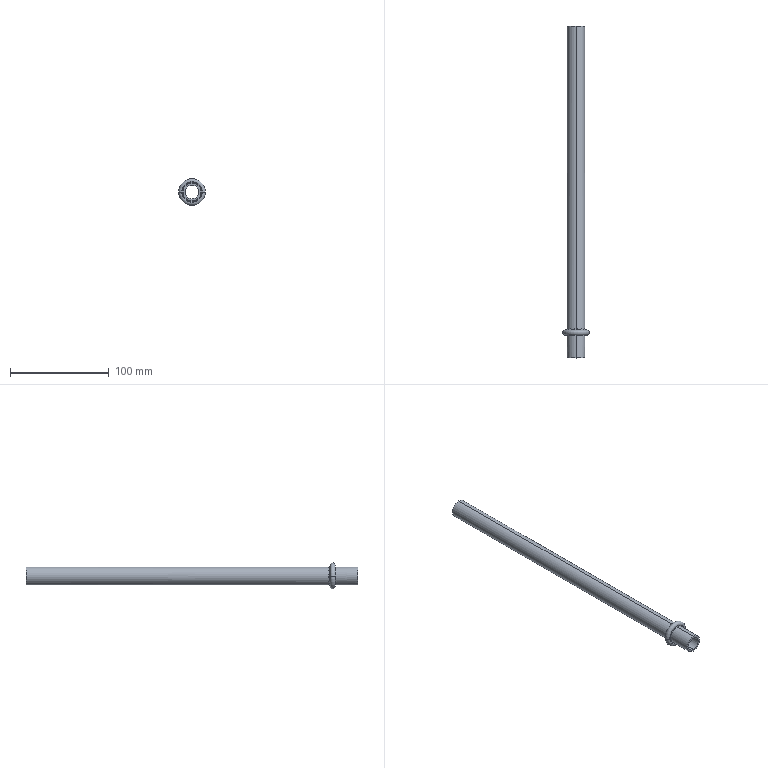Part | NX | features BREP 1 | 1 solid | 38 faces | box 27 x 335.45 x 27 mm | volume 34706 mm3 | torus 20 | cone 8 | cylinder 8 | plane 2 | commonest cylinder face diameters 14 x4 18 x4
STEP:
#1=CARTESIAN_POINT('',(-290.548,-139.151,-153.339));
#2=VERTEX_POINT('',#1);
#3=CARTESIAN_POINT('',(-289.046,-143.915,-153.339));
#4=VERTEX_POINT('',#3);
#5=CARTESIAN_POINT('',(-289.693,-141.5,-153.339));
#6=DIRECTION('',(0.,0.,1.));
#7=DIRECTION('',(1.,0.,0.));
#8=AXIS2_PLACEMENT_3D('',#5,#6,#7);
#9=CIRCLE('',#8,2.5);
#10=EDGE_CURVE('',#2,#4,#9,.T.);
#11=ORIENTED_EDGE('',*,*,#10,.T.);
#12=CARTESIAN_POINT('',(-268.34,-143.915,-153.339));
#13=VERTEX_POINT('',#12);
#14=CARTESIAN_POINT('',(-278.693,-143.915,-153.339));
#15=DIRECTION('',(0.,-1.,0.));
#16=DIRECTION('',(1.,0.,0.));
#17=AXIS2_PLACEMENT_3D('',#14,#15,#16);
#18=CIRCLE('',#17,10.353);
#19=EDGE_CURVE('',#13,#4,#18,.T.);
#20=ORIENTED_EDGE('',*,*,#19,.F.);
#21=CARTESIAN_POINT('',(-266.838,-139.151,-153.339));
#22=VERTEX_POINT('',#21);
#23=CARTESIAN_POINT('',(-267.693,-141.5,-153.339));
#24=DIRECTION('',(0.,0.,-1.));
#25=DIRECTION('',(-1.,0.,0.));
#26=AXIS2_PLACEMENT_3D('',#23,#24,#25);
#27=CIRCLE('',#26,2.5);
#28=EDGE_CURVE('',#22,#13,#27,.T.);
#29=ORIENTED_EDGE('',*,*,#28,.F.);
#30=CARTESIAN_POINT('',(-278.693,-139.151,-153.339));
#31=DIRECTION('',(0.,-1.,0.));
#32=DIRECTION('',(1.,0.,0.));
#33=AXIS2_PLACEMENT_3D('',#30,#31,#32);
#34=CIRCLE('',#33,11.855);
#35=EDGE_CURVE('',#22,#2,#34,.T.);
#36=ORIENTED_EDGE('',*,*,#35,.T.);
#37=EDGE_LOOP('',(#11,#20,#29,#36));
#38=FACE_BOUND('',#37,.T.);
#39=CARTESIAN_POINT('',(-278.693,-141.5,-153.339));
#40=DIRECTION('',(0.,-1.,0.));
#41=DIRECTION('',(-1.,0.,0.));
#42=AXIS2_PLACEMENT_3D('',#39,#40,#41);
#43=TOROIDAL_SURFACE('',#42,11.,2.5);
#44=ADVANCED_FACE('',(#38),#43,.T.);
#45=ORIENTED_EDGE('',*,*,#28,.T.);
#46=CARTESIAN_POINT('',(-278.693,-143.915,-153.339));
#47=DIRECTION('',(0.,-1.,0.));
#48=DIRECTION('',(-1.,0.,0.));
#49=AXIS2_PLACEMENT_3D('',#46,#47,#48);
#50=CIRCLE('',#49,10.353);
#51=EDGE_CURVE('',#4,#13,#50,.T.);
#52=ORIENTED_EDGE('',*,*,#51,.F.);
#53=ORIENTED_EDGE('',*,*,#10,.F.);
#54=CARTESIAN_POINT('',(-278.693,-139.151,-153.339));
#55=DIRECTION('',(0.,-1.,0.));
#56=DIRECTION('',(-1.,0.,0.));
#57=AXIS2_PLACEMENT_3D('',#54,#55,#56);
#58=CIRCLE('',#57,11.855);
#59=EDGE_CURVE('',#2,#22,#58,.T.);
#60=ORIENTED_EDGE('',*,*,#59,.T.);
#61=EDGE_LOOP('',(#45,#52,#53,#60));
#62=FACE_BOUND('',#61,.T.);
#63=CARTESIAN_POINT('',(-278.693,-141.5,-153.339));
#64=DIRECTION('',(0.,-1.,0.));
#65=DIRECTION('',(1.,0.,0.));
#66=AXIS2_PLACEMENT_3D('',#63,#64,#65);
#67=TOROIDAL_SURFACE('',#66,11.,2.5);
#68=ADVANCED_FACE('',(#62),#67,.T.);
#69=CARTESIAN_POINT('',(-288.351,-138.351,-153.339));
#70=VERTEX_POINT('',#69);
#71=CARTESIAN_POINT('',(-288.351,-138.351,-153.339));
#72=DIRECTION('',(-0.9397,-0.342,0.));
#73=VECTOR('',#72,1000.);
#74=LINE('',#71,#73);
#75=EDGE_CURVE('',#70,#2,#74,.T.);
#76=ORIENTED_EDGE('',*,*,#75,.T.);
#77=ORIENTED_EDGE('',*,*,#35,.F.);
#78=CARTESIAN_POINT('',(-269.035,-138.351,-153.339));
#79=VERTEX_POINT('',#78);
#80=CARTESIAN_POINT('',(-269.035,-138.351,-153.339));
#81=DIRECTION('',(0.9397,-0.342,0.));
#82=VECTOR('',#81,1000.);
#83=LINE('',#80,#82);
#84=EDGE_CURVE('',#79,#22,#83,.T.);
#85=ORIENTED_EDGE('',*,*,#84,.F.);
#86=CARTESIAN_POINT('',(-278.693,-138.351,-143.681));
#87=VERTEX_POINT('',#86);
#88=CARTESIAN_POINT('',(-278.693,-138.351,-153.339));
#89=DIRECTION('',(0.,-1.,0.));
#90=DIRECTION('',(1.,0.,0.));
#91=AXIS2_PLACEMENT_3D('',#88,#89,#90);
#92=CIRCLE('',#91,9.658);
#93=EDGE_CURVE('',#79,#87,#92,.T.);
#94=ORIENTED_EDGE('',*,*,#93,.T.);
#95=CARTESIAN_POINT('',(-278.693,-138.351,-153.339));
#96=DIRECTION('',(0.,-1.,0.));
#97=DIRECTION('',(0.,0.,1.));
#98=AXIS2_PLACEMENT_3D('',#95,#96,#97);
#99=CIRCLE('',#98,9.658);
#100=EDGE_CURVE('',#87,#70,#99,.T.);
#101=ORIENTED_EDGE('',*,*,#100,.T.);
#102=EDGE_LOOP('',(#76,#77,#85,#94,#101));
#103=FACE_BOUND('',#102,.T.);
#104=CARTESIAN_POINT('',(-278.693,-138.351,-153.339));
#105=DIRECTION('',(0.,-1.,0.));
#106=DIRECTION('',(0.,0.,1.));
#107=AXIS2_PLACEMENT_3D('',#104,#105,#106);
#108=CONICAL_SURFACE('',#107,9.658,1.222);
#109=ADVANCED_FACE('',(#103),#108,.T.);
#110=ORIENTED_EDGE('',*,*,#84,.T.);
#111=ORIENTED_EDGE('',*,*,#59,.F.);
#112=ORIENTED_EDGE('',*,*,#75,.F.);
#113=CARTESIAN_POINT('',(-278.693,-138.351,-162.997));
#114=VERTEX_POINT('',#113);
#115=CARTESIAN_POINT('',(-278.693,-138.351,-153.339));
#116=DIRECTION('',(0.,-1.,0.));
#117=DIRECTION('',(-1.,0.,0.));
#118=AXIS2_PLACEMENT_3D('',#115,#116,#117);
#119=CIRCLE('',#118,9.658);
#120=EDGE_CURVE('',#70,#114,#119,.T.);
#121=ORIENTED_EDGE('',*,*,#120,.T.);
#122=CARTESIAN_POINT('',(-278.693,-138.351,-153.339));
#123=DIRECTION('',(0.,-1.,0.));
#124=DIRECTION('',(0.,0.,-1.));
#125=AXIS2_PLACEMENT_3D('',#122,#123,#124);
#126=CIRCLE('',#125,9.658);
#127=EDGE_CURVE('',#114,#79,#126,.T.);
#128=ORIENTED_EDGE('',*,*,#127,.T.);
#129=EDGE_LOOP('',(#110,#111,#112,#121,#128));
#130=FACE_BOUND('',#129,.T.);
#131=CARTESIAN_POINT('',(-278.693,-138.351,-153.339));
#132=DIRECTION('',(0.,-1.,0.));
#133=DIRECTION('',(0.,0.,-1.));
#134=AXIS2_PLACEMENT_3D('',#131,#132,#133);
#135=CONICAL_SURFACE('',#134,9.658,1.222);
#136=ADVANCED_FACE('',(#130),#135,.T.);
#137=CARTESIAN_POINT('',(-278.693,-137.411,-144.339));
#138=VERTEX_POINT('',#137);
#139=CARTESIAN_POINT('',(-278.693,168.3,-144.339));
#140=VERTEX_POINT('',#139);
#141=CARTESIAN_POINT('',(-278.693,-137.411,-144.339));
#142=DIRECTION('',(0.,1.,0.));
#143=VECTOR('',#142,1000.);
#144=LINE('',#141,#143);
#145=EDGE_CURVE('',#138,#140,#144,.T.);
#146=ORIENTED_EDGE('',*,*,#145,.F.);
#147=CARTESIAN_POINT('',(-269.693,-137.411,-153.339));
#148=VERTEX_POINT('',#147);
#149=CARTESIAN_POINT('',(-278.693,-137.411,-153.339));
#150=DIRECTION('',(0.,-1.,0.));
#151=DIRECTION('',(1.,0.,0.));
#152=AXIS2_PLACEMENT_3D('',#149,#150,#151);
#153=CIRCLE('',#152,9.);
#154=EDGE_CURVE('',#148,#138,#153,.T.);
#155=ORIENTED_EDGE('',*,*,#154,.F.);
#156=CARTESIAN_POINT('',(-278.693,-137.411,-162.339));
#157=VERTEX_POINT('',#156);
#158=CARTESIAN_POINT('',(-278.693,-137.411,-153.339));
#159=DIRECTION('',(0.,-1.,0.));
#160=DIRECTION('',(0.,0.,-1.));
#161=AXIS2_PLACEMENT_3D('',#158,#159,#160);
#162=CIRCLE('',#161,9.);
#163=EDGE_CURVE('',#157,#148,#162,.T.);
#164=ORIENTED_EDGE('',*,*,#163,.F.);
#165=CARTESIAN_POINT('',(-278.693,168.3,-162.339));
#166=VERTEX_POINT('',#165);
#167=CARTESIAN_POINT('',(-278.693,-137.411,-162.339));
#168=DIRECTION('',(0.,1.,0.));
#169=VECTOR('',#168,1000.);
#170=LINE('',#167,#169);
#171=EDGE_CURVE('',#157,#166,#170,.T.);
#172=ORIENTED_EDGE('',*,*,#171,.T.);
#173=CARTESIAN_POINT('',(-278.693,168.3,-153.339));
#174=DIRECTION('',(0.,1.,0.));
#175=DIRECTION('',(0.,0.,1.));
#176=AXIS2_PLACEMENT_3D('',#173,#174,#175);
#177=CIRCLE('',#176,9.);
#178=EDGE_CURVE('',#140,#166,#177,.T.);
#179=ORIENTED_EDGE('',*,*,#178,.F.);
#180=EDGE_LOOP('',(#146,#155,#164,#172,#179));
#181=FACE_BOUND('',#180,.T.);
#182=CARTESIAN_POINT('',(-278.693,-137.411,-153.339));
#183=DIRECTION('',(0.,1.,0.));
#184=DIRECTION('',(0.,0.,-1.));
#185=AXIS2_PLACEMENT_3D('',#182,#183,#184);
#186=CYLINDRICAL_SURFACE('',#185,9.);
#187=ADVANCED_FACE('',(#181),#186,.T.);
#188=ORIENTED_EDGE('',*,*,#145,.T.);
#189=CARTESIAN_POINT('',(-278.693,168.3,-153.339));
#190=DIRECTION('',(0.,1.,0.));
#191=DIRECTION('',(0.,0.,-1.));
#192=AXIS2_PLACEMENT_3D('',#189,#190,#191);
#193=CIRCLE('',#192,9.);
#194=EDGE_CURVE('',#166,#140,#193,.T.);
#195=ORIENTED_EDGE('',*,*,#194,.F.);
#196=ORIENTED_EDGE('',*,*,#171,.F.);
#197=CARTESIAN_POINT('',(-287.693,-137.411,-153.339));
#198=VERTEX_POINT('',#197);
#199=CARTESIAN_POINT('',(-278.693,-137.411,-153.339));
#200=DIRECTION('',(0.,-1.,0.));
#201=DIRECTION('',(-1.,0.,0.));
#202=AXIS2_PLACEMENT_3D('',#199,#200,#201);
#203=CIRCLE('',#202,9.);
#204=EDGE_CURVE('',#198,#157,#203,.T.);
#205=ORIENTED_EDGE('',*,*,#204,.F.);
#206=CARTESIAN_POINT('',(-278.693,-137.411,-153.339));
#207=DIRECTION('',(0.,-1.,0.));
#208=DIRECTION('',(0.,0.,1.));
#209=AXIS2_PLACEMENT_3D('',#206,#207,#208);
#210=CIRCLE('',#209,9.);
#211=EDGE_CURVE('',#138,#198,#210,.T.);
#212=ORIENTED_EDGE('',*,*,#211,.F.);
#213=EDGE_LOOP('',(#188,#195,#196,#205,#212));
#214=FACE_BOUND('',#213,.T.);
#215=CARTESIAN_POINT('',(-278.693,-137.411,-153.339));
#216=DIRECTION('',(0.,1.,0.));
#217=DIRECTION('',(0.,0.,-1.));
#218=AXIS2_PLACEMENT_3D('',#215,#216,#217);
#219=CYLINDRICAL_SURFACE('',#218,9.);
#220=ADVANCED_FACE('',(#214),#219,.T.);
#221=CARTESIAN_POINT('',(-268.693,-137.411,-153.339));
#222=DIRECTION('',(0.,0.,1.));
#223=DIRECTION('',(0.,-1.,0.));
#224=AXIS2_PLACEMENT_3D('',#221,#222,#223);
#225=CIRCLE('',#224,1.);
#226=EDGE_CURVE('',#148,#79,#225,.T.);
#227=ORIENTED_EDGE('',*,*,#226,.F.);
#228=ORIENTED_EDGE('',*,*,#154,.T.);
#229=CARTESIAN_POINT('',(-278.693,-137.411,-143.339));
#230=DIRECTION('',(-1.,0.,0.));
#231=DIRECTION('',(0.,0.,1.));
#232=AXIS2_PLACEMENT_3D('',#229,#230,#231);
#233=CIRCLE('',#232,1.);
#234=EDGE_CURVE('',#138,#87,#233,.T.);
#235=ORIENTED_EDGE('',*,*,#234,.T.);
#236=ORIENTED_EDGE('',*,*,#93,.F.);
#237=EDGE_LOOP('',(#227,#228,#235,#236));
#238=FACE_BOUND('',#237,.T.);
#239=CARTESIAN_POINT('',(-278.693,-137.411,-153.339));
#240=DIRECTION('',(0.,1.,0.));
#241=DIRECTION('',(0.,0.,-1.));
#242=AXIS2_PLACEMENT_3D('',#239,#240,#241);
#243=TOROIDAL_SURFACE('',#242,10.,1.);
#244=ADVANCED_FACE('',(#238),#243,.F.);
#245=ORIENTED_EDGE('',*,*,#234,.F.);
#246=ORIENTED_EDGE('',*,*,#211,.T.);
#247=CARTESIAN_POINT('',(-288.693,-137.411,-153.339));
#248=DIRECTION('',(0.,0.,-1.));
#249=DIRECTION('',(0.,1.,0.));
#250=AXIS2_PLACEMENT_3D('',#247,#248,#249);
#251=CIRCLE('',#250,1.);
#252=EDGE_CURVE('',#198,#70,#251,.T.);
#253=ORIENTED_EDGE('',*,*,#252,.T.);
#254=ORIENTED_EDGE('',*,*,#100,.F.);
#255=EDGE_LOOP('',(#245,#246,#253,#254));
#256=FACE_BOUND('',#255,.T.);
#257=CARTESIAN_POINT('',(-278.693,-137.411,-153.339));
#258=DIRECTION('',(0.,-1.,0.));
#259=DIRECTION('',(0.,0.,-1.));
#260=AXIS2_PLACEMENT_3D('',#257,#258,#259);
#261=TOROIDAL_SURFACE('',#260,10.,1.);
#262=ADVANCED_FACE('',(#256),#261,.F.);
#263=ORIENTED_EDGE('',*,*,#252,.F.);
#264=ORIENTED_EDGE('',*,*,#204,.T.);
#265=CARTESIAN_POINT('',(-278.693,-137.411,-163.339));
#266=DIRECTION('',(1.,0.,0.));
#267=DIRECTION('',(0.,1.,0.));
#268=AXIS2_PLACEMENT_3D('',#265,#266,#267);
#269=CIRCLE('',#268,1.);
#270=EDGE_CURVE('',#157,#114,#269,.T.);
#271=ORIENTED_EDGE('',*,*,#270,.T.);
#272=ORIENTED_EDGE('',*,*,#120,.F.);
#273=EDGE_LOOP('',(#263,#264,#271,#272));
#274=FACE_BOUND('',#273,.T.);
#275=CARTESIAN_POINT('',(-278.693,-137.411,-153.339));
#276=DIRECTION('',(0.,1.,0.));
#277=DIRECTION('',(0.,0.,1.));
#278=AXIS2_PLACEMENT_3D('',#275,#276,#277);
#279=TOROIDAL_SURFACE('',#278,10.,1.);
#280=ADVANCED_FACE('',(#274),#279,.F.);
#281=ORIENTED_EDGE('',*,*,#270,.F.);
#282=ORIENTED_EDGE('',*,*,#163,.T.);
#283=ORIENTED_EDGE('',*,*,#226,.T.);
#284=ORIENTED_EDGE('',*,*,#127,.F.);
#285=EDGE_LOOP('',(#281,#282,#283,#284));
#286=FACE_BOUND('',#285,.T.);
#287=CARTESIAN_POINT('',(-278.693,-137.411,-153.339));
#288=DIRECTION('',(0.,1.,0.));
#289=DIRECTION('',(-1.,0.,0.));
#290=AXIS2_PLACEMENT_3D('',#287,#288,#289);
#291=TOROIDAL_SURFACE('',#290,10.,1.);
#292=ADVANCED_FACE('',(#286),#291,.F.);
#293=CARTESIAN_POINT('',(-288.071,-143.653,-153.339));
#294=VERTEX_POINT('',#293);
#295=CARTESIAN_POINT('',(-289.046,-143.915,-153.339));
#296=DIRECTION('',(0.9659,0.2588,0.));
#297=VECTOR('',#296,1000.);
#298=LINE('',#295,#297);
#299=EDGE_CURVE('',#4,#294,#298,.T.);
#300=ORIENTED_EDGE('',*,*,#299,.T.);
#301=CARTESIAN_POINT('',(-278.693,-143.653,-143.961));
#302=VERTEX_POINT('',#301);
#303=CARTESIAN_POINT('',(-278.693,-143.653,-153.339));
#304=DIRECTION('',(0.,-1.,0.));
#305=DIRECTION('',(0.,0.,1.));
#306=AXIS2_PLACEMENT_3D('',#303,#304,#305);
#307=CIRCLE('',#306,9.378);
#308=EDGE_CURVE('',#302,#294,#307,.T.);
#309=ORIENTED_EDGE('',*,*,#308,.F.);
#310=CARTESIAN_POINT('',(-269.315,-143.653,-153.339));
#311=VERTEX_POINT('',#310);
#312=CARTESIAN_POINT('',(-278.693,-143.653,-153.339));
#313=DIRECTION('',(0.,-1.,0.));
#314=DIRECTION('',(1.,0.,0.));
#315=AXIS2_PLACEMENT_3D('',#312,#313,#314);
#316=CIRCLE('',#315,9.378);
#317=EDGE_CURVE('',#311,#302,#316,.T.);
#318=ORIENTED_EDGE('',*,*,#317,.F.);
#319=CARTESIAN_POINT('',(-268.34,-143.915,-153.339));
#320=DIRECTION('',(-0.9659,0.2588,0.));
#321=VECTOR('',#320,1000.);
#322=LINE('',#319,#321);
#323=EDGE_CURVE('',#13,#311,#322,.T.);
#324=ORIENTED_EDGE('',*,*,#323,.F.);
#325=ORIENTED_EDGE('',*,*,#19,.T.);
#326=EDGE_LOOP('',(#300,#309,#318,#324,#325));
#327=FACE_BOUND('',#326,.T.);
#328=CARTESIAN_POINT('',(-278.693,-143.653,-153.339));
#329=DIRECTION('',(0.,-1.,0.));
#330=DIRECTION('',(0.,0.,1.));
#331=AXIS2_PLACEMENT_3D('',#328,#329,#330);
#332=CONICAL_SURFACE('',#331,9.378,1.309);
#333=ADVANCED_FACE('',(#327),#332,.F.);
#334=ORIENTED_EDGE('',*,*,#323,.T.);
#335=CARTESIAN_POINT('',(-278.693,-143.653,-162.717));
#336=VERTEX_POINT('',#335);
#337=CARTESIAN_POINT('',(-278.693,-143.653,-153.339));
#338=DIRECTION('',(0.,-1.,0.));
#339=DIRECTION('',(0.,0.,-1.));
#340=AXIS2_PLACEMENT_3D('',#337,#338,#339);
#341=CIRCLE('',#340,9.378);
#342=EDGE_CURVE('',#336,#311,#341,.T.);
#343=ORIENTED_EDGE('',*,*,#342,.F.);
#344=CARTESIAN_POINT('',(-278.693,-143.653,-153.339));
#345=DIRECTION('',(0.,-1.,0.));
#346=DIRECTION('',(-1.,0.,0.));
#347=AXIS2_PLACEMENT_3D('',#344,#345,#346);
#348=CIRCLE('',#347,9.378);
#349=EDGE_CURVE('',#294,#336,#348,.T.);
#350=ORIENTED_EDGE('',*,*,#349,.F.);
#351=ORIENTED_EDGE('',*,*,#299,.F.);
#352=ORIENTED_EDGE('',*,*,#51,.T.);
#353=EDGE_LOOP('',(#334,#343,#350,#351,#352));
#354=FACE_BOUND('',#353,.T.);
#355=CARTESIAN_POINT('',(-278.693,-143.653,-153.339));
#356=DIRECTION('',(0.,-1.,0.));
#357=DIRECTION('',(0.,0.,-1.));
#358=AXIS2_PLACEMENT_3D('',#355,#356,#357);
#359=CONICAL_SURFACE('',#358,9.378,1.309);
#360=ADVANCED_FACE('',(#354),#359,.F.);
#361=CARTESIAN_POINT('',(-278.693,-167.15,-144.339));
#362=VERTEX_POINT('',#361);
#363=CARTESIAN_POINT('',(-278.693,-143.943,-144.339));
#364=VERTEX_POINT('',#363);
#365=CARTESIAN_POINT('',(-278.693,-167.15,-144.339));
#366=DIRECTION('',(0.,1.,0.));
#367=VECTOR('',#366,1000.);
#368=LINE('',#365,#367);
#369=EDGE_CURVE('',#362,#364,#368,.T.);
#370=ORIENTED_EDGE('',*,*,#369,.F.);
#371=CARTESIAN_POINT('',(-278.693,-167.15,-162.339));
#372=VERTEX_POINT('',#371);
#373=CARTESIAN_POINT('',(-278.693,-167.15,-153.339));
#374=DIRECTION('',(0.,1.,0.));
#375=DIRECTION('',(0.,0.,1.));
#376=AXIS2_PLACEMENT_3D('',#373,#374,#375);
#377=CIRCLE('',#376,9.);
#378=EDGE_CURVE('',#362,#372,#377,.T.);
#379=ORIENTED_EDGE('',*,*,#378,.T.);
#380=CARTESIAN_POINT('',(-278.693,-143.943,-162.339));
#381=VERTEX_POINT('',#380);
#382=CARTESIAN_POINT('',(-278.693,-167.15,-162.339));
#383=DIRECTION('',(0.,1.,0.));
#384=VECTOR('',#383,1000.);
#385=LINE('',#382,#384);
#386=EDGE_CURVE('',#372,#381,#385,.T.);
#387=ORIENTED_EDGE('',*,*,#386,.T.);
#388=CARTESIAN_POINT('',(-269.693,-143.943,-153.339));
#389=VERTEX_POINT('',#388);
#390=CARTESIAN_POINT('',(-278.693,-143.943,-153.339));
#391=DIRECTION('',(0.,-1.,0.));
#392=DIRECTION('',(0.,0.,-1.));
#393=AXIS2_PLACEMENT_3D('',#390,#391,#392);
#394=CIRCLE('',#393,9.);
#395=EDGE_CURVE('',#381,#389,#394,.T.);
#396=ORIENTED_EDGE('',*,*,#395,.T.);
#397=CARTESIAN_POINT('',(-278.693,-143.943,-153.339));
#398=DIRECTION('',(0.,-1.,0.));
#399=DIRECTION('',(1.,0.,0.));
#400=AXIS2_PLACEMENT_3D('',#397,#398,#399);
#401=CIRCLE('',#400,9.);
#402=EDGE_CURVE('',#389,#364,#401,.T.);
#403=ORIENTED_EDGE('',*,*,#402,.T.);
#404=EDGE_LOOP('',(#370,#379,#387,#396,#403));
#405=FACE_BOUND('',#404,.T.);
#406=CARTESIAN_POINT('',(-278.693,-167.15,-153.339));
#407=DIRECTION('',(0.,1.,0.));
#408=DIRECTION('',(0.,0.,-1.));
#409=AXIS2_PLACEMENT_3D('',#406,#407,#408);
#410=CYLINDRICAL_SURFACE('',#409,9.);
#411=ADVANCED_FACE('',(#405),#410,.T.);
#412=ORIENTED_EDGE('',*,*,#369,.T.);
#413=CARTESIAN_POINT('',(-287.693,-143.943,-153.339));
#414=VERTEX_POINT('',#413);
#415=CARTESIAN_POINT('',(-278.693,-143.943,-153.339));
#416=DIRECTION('',(0.,-1.,0.));
#417=DIRECTION('',(0.,0.,1.));
#418=AXIS2_PLACEMENT_3D('',#415,#416,#417);
#419=CIRCLE('',#418,9.);
#420=EDGE_CURVE('',#364,#414,#419,.T.);
#421=ORIENTED_EDGE('',*,*,#420,.T.);
#422=CARTESIAN_POINT('',(-278.693,-143.943,-153.339));
#423=DIRECTION('',(0.,-1.,0.));
#424=DIRECTION('',(-1.,0.,0.));
#425=AXIS2_PLACEMENT_3D('',#422,#423,#424);
#426=CIRCLE('',#425,9.);
#427=EDGE_CURVE('',#414,#381,#426,.T.);
#428=ORIENTED_EDGE('',*,*,#427,.T.);
#429=ORIENTED_EDGE('',*,*,#386,.F.);
#430=CARTESIAN_POINT('',(-278.693,-167.15,-153.339));
#431=DIRECTION('',(0.,1.,0.));
#432=DIRECTION('',(0.,0.,-1.));
#433=AXIS2_PLACEMENT_3D('',#430,#431,#432);
#434=CIRCLE('',#433,9.);
#435=EDGE_CURVE('',#372,#362,#434,.T.);
#436=ORIENTED_EDGE('',*,*,#435,.T.);
#437=EDGE_LOOP('',(#412,#421,#428,#429,#436));
#438=FACE_BOUND('',#437,.T.);
#439=CARTESIAN_POINT('',(-278.693,-167.15,-153.339));
#440=DIRECTION('',(0.,1.,0.));
#441=DIRECTION('',(0.,0.,-1.));
#442=AXIS2_PLACEMENT_3D('',#439,#440,#441);
#443=CYLINDRICAL_SURFACE('',#442,9.);
#444=ADVANCED_FACE('',(#438),#443,.T.);
#445=CARTESIAN_POINT('',(-269.393,-143.943,-153.339));
#446=DIRECTION('',(0.,0.,-1.));
#447=DIRECTION('',(-1.,0.,0.));
#448=AXIS2_PLACEMENT_3D('',#445,#446,#447);
#449=CIRCLE('',#448,0.3);
#450=EDGE_CURVE('',#311,#389,#449,.F.);
#451=ORIENTED_EDGE('',*,*,#450,.F.);
#452=ORIENTED_EDGE('',*,*,#317,.T.);
#453=CARTESIAN_POINT('',(-278.693,-143.943,-144.039));
#454=DIRECTION('',(1.,0.,0.));
#455=DIRECTION('',(0.,0.,-1.));
#456=AXIS2_PLACEMENT_3D('',#453,#454,#455);
#457=CIRCLE('',#456,0.3);
#458=EDGE_CURVE('',#302,#364,#457,.F.);
#459=ORIENTED_EDGE('',*,*,#458,.T.);
#460=ORIENTED_EDGE('',*,*,#402,.F.);
#461=EDGE_LOOP('',(#451,#452,#459,#460));
#462=FACE_BOUND('',#461,.T.);
#463=CARTESIAN_POINT('',(-278.693,-143.943,-153.339));
#464=DIRECTION('',(0.,-1.,0.));
#465=DIRECTION('',(-1.,0.,0.));
#466=AXIS2_PLACEMENT_3D('',#463,#464,#465);
#467=TOROIDAL_SURFACE('',#466,9.3,0.3);
#468=ADVANCED_FACE('',(#462),#467,.F.);
#469=ORIENTED_EDGE('',*,*,#458,.F.);
#470=ORIENTED_EDGE('',*,*,#308,.T.);
#471=CARTESIAN_POINT('',(-287.993,-143.943,-153.339));
#472=DIRECTION('',(0.,0.,1.));
#473=DIRECTION('',(1.,0.,0.));
#474=AXIS2_PLACEMENT_3D('',#471,#472,#473);
#475=CIRCLE('',#474,0.3);
#476=EDGE_CURVE('',#294,#414,#475,.F.);
#477=ORIENTED_EDGE('',*,*,#476,.T.);
#478=ORIENTED_EDGE('',*,*,#420,.F.);
#479=EDGE_LOOP('',(#469,#470,#477,#478));
#480=FACE_BOUND('',#479,.T.);
#481=CARTESIAN_POINT('',(-278.693,-143.943,-153.339));
#482=DIRECTION('',(0.,-1.,0.));
#483=DIRECTION('',(0.,0.,-1.));
#484=AXIS2_PLACEMENT_3D('',#481,#482,#483);
#485=TOROIDAL_SURFACE('',#484,9.3,0.3);
#486=ADVANCED_FACE('',(#480),#485,.F.);
#487=ORIENTED_EDGE('',*,*,#476,.F.);
#488=ORIENTED_EDGE('',*,*,#349,.T.);
#489=CARTESIAN_POINT('',(-278.693,-143.943,-162.639));
#490=DIRECTION('',(-1.,0.,0.));
#491=DIRECTION('',(0.,0.,1.));
#492=AXIS2_PLACEMENT_3D('',#489,#490,#491);
#493=CIRCLE('',#492,0.3);
#494=EDGE_CURVE('',#336,#381,#493,.F.);
#495=ORIENTED_EDGE('',*,*,#494,.T.);
#496=ORIENTED_EDGE('',*,*,#427,.F.);
#497=EDGE_LOOP('',(#487,#488,#495,#496));
#498=FACE_BOUND('',#497,.T.);
#499=CARTESIAN_POINT('',(-278.693,-143.943,-153.339));
#500=DIRECTION('',(0.,-1.,0.));
#501=DIRECTION('',(1.,0.,0.));
#502=AXIS2_PLACEMENT_3D('',#499,#500,#501);
#503=TOROIDAL_SURFACE('',#502,9.3,0.3);
#504=ADVANCED_FACE('',(#498),#503,.F.);
#505=ORIENTED_EDGE('',*,*,#494,.F.);
#506=ORIENTED_EDGE('',*,*,#342,.T.);
#507=ORIENTED_EDGE('',*,*,#450,.T.);
#508=ORIENTED_EDGE('',*,*,#395,.F.);
#509=EDGE_LOOP('',(#505,#506,#507,#508));
#510=FACE_BOUND('',#509,.T.);
#511=CARTESIAN_POINT('',(-278.693,-143.943,-153.339));
#512=DIRECTION('',(0.,-1.,0.));
#513=DIRECTION('',(0.,0.,1.));
#514=AXIS2_PLACEMENT_3D('',#511,#512,#513);
#515=TOROIDAL_SURFACE('',#514,9.3,0.3);
#516=ADVANCED_FACE('',(#510),#515,.F.);
#517=ORIENTED_EDGE('',*,*,#178,.T.);
#518=ORIENTED_EDGE('',*,*,#194,.T.);
#519=EDGE_LOOP('',(#517,#518));
#520=FACE_BOUND('',#519,.T.);
#521=CARTESIAN_POINT('',(-278.693,168.3,-160.339));
#522=VERTEX_POINT('',#521);
#523=CARTESIAN_POINT('',(-278.693,168.3,-146.339));
#524=VERTEX_POINT('',#523);
#525=CARTESIAN_POINT('',(-278.693,168.3,-153.339));
#526=DIRECTION('',(0.,-1.,0.));
#527=DIRECTION('',(0.,0.,-1.));
#528=AXIS2_PLACEMENT_3D('',#525,#526,#527);
#529=CIRCLE('',#528,7.);
#530=EDGE_CURVE('',#522,#524,#529,.T.);
#531=ORIENTED_EDGE('',*,*,#530,.T.);
#532=CARTESIAN_POINT('',(-278.693,168.3,-153.339));
#533=DIRECTION('',(0.,-1.,0.));
#534=DIRECTION('',(0.,0.,1.));
#535=AXIS2_PLACEMENT_3D('',#532,#533,#534);
#536=CIRCLE('',#535,7.);
#537=EDGE_CURVE('',#524,#522,#536,.T.);
#538=ORIENTED_EDGE('',*,*,#537,.T.);
#539=EDGE_LOOP('',(#531,#538));
#540=FACE_BOUND('',#539,.T.);
#541=CARTESIAN_POINT('',(-294.893,168.3,-164.139));
#542=DIRECTION('',(0.,1.,0.));
#543=DIRECTION('',(-1.,0.,0.));
#544=AXIS2_PLACEMENT_3D('',#541,#542,#543);
#545=PLANE('',#544);
#546=ADVANCED_FACE('',(#520,#540),#545,.T.);
#547=ORIENTED_EDGE('',*,*,#378,.F.);
#548=ORIENTED_EDGE('',*,*,#435,.F.);
#549=EDGE_LOOP('',(#547,#548));
#550=FACE_BOUND('',#549,.T.);
#551=CARTESIAN_POINT('',(-278.693,-167.15,-160.339));
#552=VERTEX_POINT('',#551);
#553=CARTESIAN_POINT('',(-278.693,-167.15,-146.339));
#554=VERTEX_POINT('',#553);
#555=CARTESIAN_POINT('',(-278.693,-167.15,-153.339));
#556=DIRECTION('',(0.,1.,0.));
#557=DIRECTION('',(0.,0.,-1.));
#558=AXIS2_PLACEMENT_3D('',#555,#556,#557);
#559=CIRCLE('',#558,7.);
#560=EDGE_CURVE('',#552,#554,#559,.T.);
#561=ORIENTED_EDGE('',*,*,#560,.T.);
#562=CARTESIAN_POINT('',(-278.693,-167.15,-153.339));
#563=DIRECTION('',(0.,1.,0.));
#564=DIRECTION('',(0.,0.,1.));
#565=AXIS2_PLACEMENT_3D('',#562,#563,#564);
#566=CIRCLE('',#565,7.);
#567=EDGE_CURVE('',#554,#552,#566,.T.);
#568=ORIENTED_EDGE('',*,*,#567,.T.);
#569=EDGE_LOOP('',(#561,#568));
#570=FACE_BOUND('',#569,.T.);
#571=CARTESIAN_POINT('',(-294.893,-167.15,-164.139));
#572=DIRECTION('',(0.,-1.,0.));
#573=DIRECTION('',(0.,0.,1.));
#574=AXIS2_PLACEMENT_3D('',#571,#572,#573);
#575=PLANE('',#574);
#576=ADVANCED_FACE('',(#550,#570),#575,.T.);
#577=CARTESIAN_POINT('',(-271.693,-137.411,-153.339));
#578=VERTEX_POINT('',#577);
#579=CARTESIAN_POINT('',(-278.693,-137.411,-160.339));
#580=VERTEX_POINT('',#579);
#581=CARTESIAN_POINT('',(-278.693,-137.411,-160.339));
#582=CARTESIAN_POINT('',(-276.86,-137.411,-160.339));
#583=CARTESIAN_POINT('',(-273.21,-137.411,-158.822));
#584=CARTESIAN_POINT('',(-271.693,-137.411,-155.172));
#585=CARTESIAN_POINT('',(-271.693,-137.411,-153.339));
#586=B_SPLINE_CURVE_WITH_KNOTS('',3,(#581,#582,#583,#584,#585),.UNSPECIFIED.,.F.,.F.,(4,1,4),(0.,0.5,1.),.UNSPECIFIED.);
#587=EDGE_CURVE('',#578,#580,#586,.F.);
#588=ORIENTED_EDGE('',*,*,#587,.T.);
#589=CARTESIAN_POINT('',(-278.693,-140.23,-162.313));
#590=VERTEX_POINT('',#589);
#591=CARTESIAN_POINT('',(-278.693,-140.23,-162.313));
#592=CARTESIAN_POINT('',(-278.693,-139.813,-161.165));
#593=CARTESIAN_POINT('',(-278.693,-138.633,-160.339));
#594=CARTESIAN_POINT('',(-278.693,-137.411,-160.339));
#595=B_SPLINE_CURVE_WITH_KNOTS('',3,(#591,#592,#593,#594),.UNSPECIFIED.,.F.,.F.,(4,4),(0.,1.),.UNSPECIFIED.);
#596=EDGE_CURVE('',#590,#580,#595,.T.);
#597=ORIENTED_EDGE('',*,*,#596,.F.);
#598=CARTESIAN_POINT('',(-269.719,-140.23,-153.339));
#599=VERTEX_POINT('',#598);
#600=CARTESIAN_POINT('',(-278.693,-140.23,-162.313));
#601=CARTESIAN_POINT('',(-276.344,-140.23,-162.313));
#602=CARTESIAN_POINT('',(-271.664,-140.23,-160.368));
#603=CARTESIAN_POINT('',(-269.719,-140.23,-155.688));
#604=CARTESIAN_POINT('',(-269.719,-140.23,-153.339));
#605=B_SPLINE_CURVE_WITH_KNOTS('',3,(#600,#601,#602,#603,#604),.UNSPECIFIED.,.F.,.F.,(4,1,4),(0.,0.5,1.),.UNSPECIFIED.);
#606=EDGE_CURVE('',#599,#590,#605,.F.);
#607=ORIENTED_EDGE('',*,*,#606,.F.);
#608=CARTESIAN_POINT('',(-269.719,-140.23,-153.339));
#609=CARTESIAN_POINT('',(-270.867,-139.813,-153.339));
#610=CARTESIAN_POINT('',(-271.693,-138.633,-153.339));
#611=CARTESIAN_POINT('',(-271.693,-137.411,-153.339));
#612=B_SPLINE_CURVE_WITH_KNOTS('',3,(#608,#609,#610,#611),.UNSPECIFIED.,.F.,.F.,(4,4),(0.,1.),.UNSPECIFIED.);
#613=EDGE_CURVE('',#599,#578,#612,.T.);
#614=ORIENTED_EDGE('',*,*,#613,.T.);
#615=EDGE_LOOP('',(#588,#597,#607,#614));
#616=FACE_BOUND('',#615,.T.);
#617=CARTESIAN_POINT('',(-278.694,-137.411,-153.338));
#618=DIRECTION('',(0.,1.,0.));
#619=DIRECTION('',(-1.,0.,0.00006098));
#620=AXIS2_PLACEMENT_3D('',#617,#618,#619);
#621=TOROIDAL_SURFACE('',#620,10.001,3.);
#622=ADVANCED_FACE('',(#616),#621,.T.);
#623=CARTESIAN_POINT('',(-278.693,-137.411,-146.339));
#624=VERTEX_POINT('',#623);
#625=CARTESIAN_POINT('',(-278.693,-137.411,-146.339));
#626=DIRECTION('',(0.,1.,0.));
#627=VECTOR('',#626,1000.);
#628=LINE('',#625,#627);
#629=EDGE_CURVE('',#524,#624,#628,.F.);
#630=ORIENTED_EDGE('',*,*,#629,.F.);
#631=ORIENTED_EDGE('',*,*,#530,.F.);
#632=CARTESIAN_POINT('',(-278.693,-137.411,-160.339));
#633=DIRECTION('',(0.,1.,0.));
#634=VECTOR('',#633,1000.);
#635=LINE('',#632,#634);
#636=EDGE_CURVE('',#522,#580,#635,.F.);
#637=ORIENTED_EDGE('',*,*,#636,.T.);
#638=ORIENTED_EDGE('',*,*,#587,.F.);
#639=CARTESIAN_POINT('',(-271.693,-137.411,-153.339));
#640=CARTESIAN_POINT('',(-271.693,-137.411,-151.506));
#641=CARTESIAN_POINT('',(-273.21,-137.411,-147.856));
#642=CARTESIAN_POINT('',(-276.86,-137.411,-146.339));
#643=CARTESIAN_POINT('',(-278.693,-137.411,-146.339));
#644=B_SPLINE_CURVE_WITH_KNOTS('',3,(#639,#640,#641,#642,#643),.UNSPECIFIED.,.F.,.F.,(4,1,4),(0.,0.5,1.),.UNSPECIFIED.);
#645=EDGE_CURVE('',#624,#578,#644,.F.);
#646=ORIENTED_EDGE('',*,*,#645,.F.);
#647=EDGE_LOOP('',(#630,#631,#637,#638,#646));
#648=FACE_BOUND('',#647,.T.);
#649=CARTESIAN_POINT('',(-278.693,-137.411,-153.339));
#650=DIRECTION('',(0.,1.,0.));
#651=DIRECTION('',(0.,0.,-1.));
#652=AXIS2_PLACEMENT_3D('',#649,#650,#651);
#653=CYLINDRICAL_SURFACE('',#652,7.);
#654=ADVANCED_FACE('',(#648),#653,.F.);
#655=CARTESIAN_POINT('',(-287.667,-140.23,-153.339));
#656=VERTEX_POINT('',#655);
#657=CARTESIAN_POINT('',(-285.693,-137.411,-153.339));
#658=VERTEX_POINT('',#657);
#659=CARTESIAN_POINT('',(-287.667,-140.23,-153.339));
#660=CARTESIAN_POINT('',(-286.519,-139.813,-153.339));
#661=CARTESIAN_POINT('',(-285.693,-138.633,-153.339));
#662=CARTESIAN_POINT('',(-285.693,-137.411,-153.339));
#663=B_SPLINE_CURVE_WITH_KNOTS('',3,(#659,#660,#661,#662),.UNSPECIFIED.,.F.,.F.,(4,4),(0.,1.),.UNSPECIFIED.);
#664=EDGE_CURVE('',#656,#658,#663,.T.);
#665=ORIENTED_EDGE('',*,*,#664,.F.);
#666=CARTESIAN_POINT('',(-287.667,-140.23,-153.339));
#667=CARTESIAN_POINT('',(-287.667,-140.23,-155.688));
#668=CARTESIAN_POINT('',(-285.722,-140.23,-160.368));
#669=CARTESIAN_POINT('',(-281.042,-140.23,-162.313));
#670=CARTESIAN_POINT('',(-278.693,-140.23,-162.313));
#671=B_SPLINE_CURVE_WITH_KNOTS('',3,(#666,#667,#668,#669,#670),.UNSPECIFIED.,.F.,.F.,(4,1,4),(0.,0.5,1.),.UNSPECIFIED.);
#672=EDGE_CURVE('',#590,#656,#671,.F.);
#673=ORIENTED_EDGE('',*,*,#672,.F.);
#674=ORIENTED_EDGE('',*,*,#596,.T.);
#675=CARTESIAN_POINT('',(-285.693,-137.411,-153.339));
#676=CARTESIAN_POINT('',(-285.693,-137.411,-155.172));
#677=CARTESIAN_POINT('',(-284.176,-137.411,-158.822));
#678=CARTESIAN_POINT('',(-280.526,-137.411,-160.339));
#679=CARTESIAN_POINT('',(-278.693,-137.411,-160.339));
#680=B_SPLINE_CURVE_WITH_KNOTS('',3,(#675,#676,#677,#678,#679),.UNSPECIFIED.,.F.,.F.,(4,1,4),(0.,0.5,1.),.UNSPECIFIED.);
#681=EDGE_CURVE('',#580,#658,#680,.F.);
#682=ORIENTED_EDGE('',*,*,#681,.T.);
#683=EDGE_LOOP('',(#665,#673,#674,#682));
#684=FACE_BOUND('',#683,.T.);
#685=CARTESIAN_POINT('',(-278.692,-137.411,-153.338));
#686=DIRECTION('',(0.,1.,0.));
#687=DIRECTION('',(0.00006098,0.,1.));
#688=AXIS2_PLACEMENT_3D('',#685,#686,#687);
#689=TOROIDAL_SURFACE('',#688,10.001,3.);
#690=ADVANCED_FACE('',(#684),#689,.T.);
#691=ORIENTED_EDGE('',*,*,#606,.T.);
#692=ORIENTED_EDGE('',*,*,#672,.T.);
#693=CARTESIAN_POINT('',(-289.864,-141.03,-153.339));
#694=VERTEX_POINT('',#693);
#695=CARTESIAN_POINT('',(-289.864,-141.03,-153.339));
#696=DIRECTION('',(0.9397,0.342,0.));
#697=VECTOR('',#696,1000.);
#698=LINE('',#695,#697);
#699=EDGE_CURVE('',#656,#694,#698,.F.);
#700=ORIENTED_EDGE('',*,*,#699,.T.);
#701=CARTESIAN_POINT('',(-267.522,-141.03,-153.339));
#702=VERTEX_POINT('',#701);
#703=CARTESIAN_POINT('',(-278.693,-141.03,-153.339));
#704=DIRECTION('',(0.,-1.,0.));
#705=DIRECTION('',(-1.,0.,0.));
#706=AXIS2_PLACEMENT_3D('',#703,#704,#705);
#707=CIRCLE('',#706,11.171);
#708=EDGE_CURVE('',#694,#702,#707,.T.);
#709=ORIENTED_EDGE('',*,*,#708,.T.);
#710=CARTESIAN_POINT('',(-267.522,-141.03,-153.339));
#711=DIRECTION('',(-0.9397,0.342,0.));
#712=VECTOR('',#711,1000.);
#713=LINE('',#710,#712);
#714=EDGE_CURVE('',#599,#702,#713,.F.);
#715=ORIENTED_EDGE('',*,*,#714,.F.);
#716=EDGE_LOOP('',(#691,#692,#700,#709,#715));
#717=FACE_BOUND('',#716,.T.);
#718=CARTESIAN_POINT('',(-278.693,-140.23,-153.339));
#719=DIRECTION('',(0.,-1.,0.));
#720=DIRECTION('',(0.,0.,-1.));
#721=AXIS2_PLACEMENT_3D('',#718,#719,#720);
#722=CONICAL_SURFACE('',#721,8.974,1.222);
#723=ADVANCED_FACE('',(#717),#722,.F.);
#724=ORIENTED_EDGE('',*,*,#613,.F.);
#725=CARTESIAN_POINT('',(-278.693,-140.23,-144.365));
#726=VERTEX_POINT('',#725);
#727=CARTESIAN_POINT('',(-269.719,-140.23,-153.339));
#728=CARTESIAN_POINT('',(-269.719,-140.23,-150.99));
#729=CARTESIAN_POINT('',(-271.664,-140.23,-146.31));
#730=CARTESIAN_POINT('',(-276.344,-140.23,-144.365));
#731=CARTESIAN_POINT('',(-278.693,-140.23,-144.365));
#732=B_SPLINE_CURVE_WITH_KNOTS('',3,(#727,#728,#729,#730,#731),.UNSPECIFIED.,.F.,.F.,(4,1,4),(0.,0.5,1.),.UNSPECIFIED.);
#733=EDGE_CURVE('',#726,#599,#732,.F.);
#734=ORIENTED_EDGE('',*,*,#733,.F.);
#735=CARTESIAN_POINT('',(-278.693,-140.23,-144.365));
#736=CARTESIAN_POINT('',(-278.693,-139.813,-145.513));
#737=CARTESIAN_POINT('',(-278.693,-138.633,-146.339));
#738=CARTESIAN_POINT('',(-278.693,-137.411,-146.339));
#739=B_SPLINE_CURVE_WITH_KNOTS('',3,(#735,#736,#737,#738),.UNSPECIFIED.,.F.,.F.,(4,4),(0.,1.),.UNSPECIFIED.);
#740=EDGE_CURVE('',#726,#624,#739,.T.);
#741=ORIENTED_EDGE('',*,*,#740,.T.);
#742=ORIENTED_EDGE('',*,*,#645,.T.);
#743=EDGE_LOOP('',(#724,#734,#741,#742));
#744=FACE_BOUND('',#743,.T.);
#745=CARTESIAN_POINT('',(-278.694,-137.411,-153.34));
#746=DIRECTION('',(0.,1.,0.));
#747=DIRECTION('',(-0.00006098,0.,-1.));
#748=AXIS2_PLACEMENT_3D('',#745,#746,#747);
#749=TOROIDAL_SURFACE('',#748,10.001,3.);
#750=ADVANCED_FACE('',(#744),#749,.T.);
#751=ORIENTED_EDGE('',*,*,#629,.T.);
#752=CARTESIAN_POINT('',(-278.693,-137.411,-146.339));
#753=CARTESIAN_POINT('',(-280.526,-137.411,-146.339));
#754=CARTESIAN_POINT('',(-284.176,-137.411,-147.856));
#755=CARTESIAN_POINT('',(-285.693,-137.411,-151.506));
#756=CARTESIAN_POINT('',(-285.693,-137.411,-153.339));
#757=B_SPLINE_CURVE_WITH_KNOTS('',3,(#752,#753,#754,#755,#756),.UNSPECIFIED.,.F.,.F.,(4,1,4),(0.,0.5,1.),.UNSPECIFIED.);
#758=EDGE_CURVE('',#624,#658,#757,.T.);
#759=ORIENTED_EDGE('',*,*,#758,.T.);
#760=ORIENTED_EDGE('',*,*,#681,.F.);
#761=ORIENTED_EDGE('',*,*,#636,.F.);
#762=ORIENTED_EDGE('',*,*,#537,.F.);
#763=EDGE_LOOP('',(#751,#759,#760,#761,#762));
#764=FACE_BOUND('',#763,.T.);
#765=CARTESIAN_POINT('',(-278.693,-137.411,-153.339));
#766=DIRECTION('',(0.,1.,0.));
#767=DIRECTION('',(0.,0.,-1.));
#768=AXIS2_PLACEMENT_3D('',#765,#766,#767);
#769=CYLINDRICAL_SURFACE('',#768,7.);
#770=ADVANCED_FACE('',(#764),#769,.F.);
#771=ORIENTED_EDGE('',*,*,#758,.F.);
#772=ORIENTED_EDGE('',*,*,#740,.F.);
#773=CARTESIAN_POINT('',(-278.693,-140.23,-144.365));
#774=CARTESIAN_POINT('',(-281.042,-140.23,-144.365));
#775=CARTESIAN_POINT('',(-285.722,-140.23,-146.31));
#776=CARTESIAN_POINT('',(-287.667,-140.23,-150.99));
#777=CARTESIAN_POINT('',(-287.667,-140.23,-153.339));
#778=B_SPLINE_CURVE_WITH_KNOTS('',3,(#773,#774,#775,#776,#777),.UNSPECIFIED.,.F.,.F.,(4,1,4),(0.,0.5,1.),.UNSPECIFIED.);
#779=EDGE_CURVE('',#726,#656,#778,.T.);
#780=ORIENTED_EDGE('',*,*,#779,.T.);
#781=ORIENTED_EDGE('',*,*,#664,.T.);
#782=EDGE_LOOP('',(#771,#772,#780,#781));
#783=FACE_BOUND('',#782,.T.);
#784=CARTESIAN_POINT('',(-278.692,-137.411,-153.34));
#785=DIRECTION('',(0.,-1.,0.));
#786=DIRECTION('',(0.00006098,0.,-1.));
#787=AXIS2_PLACEMENT_3D('',#784,#785,#786);
#788=TOROIDAL_SURFACE('',#787,10.001,3.);
#789=ADVANCED_FACE('',(#783),#788,.T.);
#790=ORIENTED_EDGE('',*,*,#699,.F.);
#791=ORIENTED_EDGE('',*,*,#779,.F.);
#792=ORIENTED_EDGE('',*,*,#733,.T.);
#793=ORIENTED_EDGE('',*,*,#714,.T.);
#794=CARTESIAN_POINT('',(-278.693,-141.03,-153.339));
#795=DIRECTION('',(0.,-1.,0.));
#796=DIRECTION('',(1.,0.,0.));
#797=AXIS2_PLACEMENT_3D('',#794,#795,#796);
#798=CIRCLE('',#797,11.171);
#799=EDGE_CURVE('',#702,#694,#798,.T.);
#800=ORIENTED_EDGE('',*,*,#799,.T.);
#801=EDGE_LOOP('',(#790,#791,#792,#793,#800));
#802=FACE_BOUND('',#801,.T.);
#803=CARTESIAN_POINT('',(-278.693,-140.23,-153.339));
#804=DIRECTION('',(0.,-1.,0.));
#805=DIRECTION('',(0.,0.,1.));
#806=AXIS2_PLACEMENT_3D('',#803,#804,#805);
#807=CONICAL_SURFACE('',#806,8.974,1.222);
#808=ADVANCED_FACE('',(#802),#807,.F.);
#809=CARTESIAN_POINT('',(-267.822,-141.983,-153.339));
#810=VERTEX_POINT('',#809);
#811=CARTESIAN_POINT('',(-267.693,-141.5,-153.339));
#812=DIRECTION('',(0.,0.,-1.));
#813=DIRECTION('',(-1.,0.,0.));
#814=AXIS2_PLACEMENT_3D('',#811,#812,#813);
#815=CIRCLE('',#814,0.5);
#816=EDGE_CURVE('',#702,#810,#815,.T.);
#817=ORIENTED_EDGE('',*,*,#816,.F.);
#818=ORIENTED_EDGE('',*,*,#708,.F.);
#819=CARTESIAN_POINT('',(-289.564,-141.983,-153.339));
#820=VERTEX_POINT('',#819);
#821=CARTESIAN_POINT('',(-289.693,-141.5,-153.339));
#822=DIRECTION('',(0.,0.,1.));
#823=DIRECTION('',(1.,0.,0.));
#824=AXIS2_PLACEMENT_3D('',#821,#822,#823);
#825=CIRCLE('',#824,0.5);
#826=EDGE_CURVE('',#694,#820,#825,.T.);
#827=ORIENTED_EDGE('',*,*,#826,.T.);
#828=CARTESIAN_POINT('',(-278.693,-141.983,-153.339));
#829=DIRECTION('',(0.,-1.,0.));
#830=DIRECTION('',(-1.,0.,0.));
#831=AXIS2_PLACEMENT_3D('',#828,#829,#830);
#832=CIRCLE('',#831,10.871);
#833=EDGE_CURVE('',#820,#810,#832,.T.);
#834=ORIENTED_EDGE('',*,*,#833,.T.);
#835=EDGE_LOOP('',(#817,#818,#827,#834));
#836=FACE_BOUND('',#835,.T.);
#837=CARTESIAN_POINT('',(-278.693,-141.5,-153.339));
#838=DIRECTION('',(0.,-1.,0.));
#839=DIRECTION('',(1.,0.,0.));
#840=AXIS2_PLACEMENT_3D('',#837,#838,#839);
#841=TOROIDAL_SURFACE('',#840,11.,0.5);
#842=ADVANCED_FACE('',(#836),#841,.F.);
#843=CARTESIAN_POINT('',(-278.693,-141.983,-153.339));
#844=DIRECTION('',(0.,-1.,0.));
#845=DIRECTION('',(1.,0.,0.));
#846=AXIS2_PLACEMENT_3D('',#843,#844,#845);
#847=CIRCLE('',#846,10.871);
#848=EDGE_CURVE('',#810,#820,#847,.T.);
#849=ORIENTED_EDGE('',*,*,#848,.T.);
#850=ORIENTED_EDGE('',*,*,#826,.F.);
#851=ORIENTED_EDGE('',*,*,#799,.F.);
#852=ORIENTED_EDGE('',*,*,#816,.T.);
#853=EDGE_LOOP('',(#849,#850,#851,#852));
#854=FACE_BOUND('',#853,.T.);
#855=CARTESIAN_POINT('',(-278.693,-141.5,-153.339));
#856=DIRECTION('',(0.,-1.,0.));
#857=DIRECTION('',(-1.,0.,0.));
#858=AXIS2_PLACEMENT_3D('',#855,#856,#857);
#859=TOROIDAL_SURFACE('',#858,11.,0.5);
#860=ADVANCED_FACE('',(#854),#859,.F.);
#861=CARTESIAN_POINT('',(-288.588,-141.722,-153.339));
#862=VERTEX_POINT('',#861);
#863=CARTESIAN_POINT('',(-278.693,-141.722,-163.234));
#864=VERTEX_POINT('',#863);
#865=CARTESIAN_POINT('',(-278.693,-141.722,-163.234));
#866=CARTESIAN_POINT('',(-281.284,-141.722,-163.234));
#867=CARTESIAN_POINT('',(-286.444,-141.722,-161.09));
#868=CARTESIAN_POINT('',(-288.588,-141.722,-155.93));
#869=CARTESIAN_POINT('',(-288.588,-141.722,-153.339));
#870=B_SPLINE_CURVE_WITH_KNOTS('',3,(#865,#866,#867,#868,#869),.UNSPECIFIED.,.F.,.F.,(4,1,4),(0.,0.5,1.),.UNSPECIFIED.);
#871=EDGE_CURVE('',#862,#864,#870,.F.);
#872=ORIENTED_EDGE('',*,*,#871,.T.);
#873=CARTESIAN_POINT('',(-268.798,-141.722,-153.339));
#874=VERTEX_POINT('',#873);
#875=CARTESIAN_POINT('',(-268.798,-141.722,-153.339));
#876=CARTESIAN_POINT('',(-268.798,-141.722,-155.93));
#877=CARTESIAN_POINT('',(-270.942,-141.722,-161.09));
#878=CARTESIAN_POINT('',(-276.102,-141.722,-163.234));
#879=CARTESIAN_POINT('',(-278.693,-141.722,-163.234));
#880=B_SPLINE_CURVE_WITH_KNOTS('',3,(#875,#876,#877,#878,#879),.UNSPECIFIED.,.F.,.F.,(4,1,4),(0.,0.5,1.),.UNSPECIFIED.);
#881=EDGE_CURVE('',#864,#874,#880,.F.);
#882=ORIENTED_EDGE('',*,*,#881,.T.);
#883=CARTESIAN_POINT('',(-267.822,-141.983,-153.339));
#884=DIRECTION('',(-0.9659,0.2588,0.));
#885=VECTOR('',#884,1000.);
#886=LINE('',#883,#885);
#887=EDGE_CURVE('',#810,#874,#886,.T.);
#888=ORIENTED_EDGE('',*,*,#887,.F.);
#889=ORIENTED_EDGE('',*,*,#833,.F.);
#890=CARTESIAN_POINT('',(-289.564,-141.983,-153.339));
#891=DIRECTION('',(0.9659,0.2588,0.));
#892=VECTOR('',#891,1000.);
#893=LINE('',#890,#892);
#894=EDGE_CURVE('',#820,#862,#893,.T.);
#895=ORIENTED_EDGE('',*,*,#894,.T.);
#896=EDGE_LOOP('',(#872,#882,#888,#889,#895));
#897=FACE_BOUND('',#896,.T.);
#898=CARTESIAN_POINT('',(-278.693,-141.722,-153.339));
#899=DIRECTION('',(0.,-1.,0.));
#900=DIRECTION('',(0.,0.,-1.));
#901=AXIS2_PLACEMENT_3D('',#898,#899,#900);
#902=CONICAL_SURFACE('',#901,9.895,1.309);
#903=ADVANCED_FACE('',(#897),#902,.T.);
#904=CARTESIAN_POINT('',(-278.693,-141.722,-143.444));
#905=VERTEX_POINT('',#904);
#906=CARTESIAN_POINT('',(-278.693,-141.722,-143.444));
#907=CARTESIAN_POINT('',(-276.102,-141.722,-143.444));
#908=CARTESIAN_POINT('',(-270.942,-141.722,-145.588));
#909=CARTESIAN_POINT('',(-268.798,-141.722,-150.748));
#910=CARTESIAN_POINT('',(-268.798,-141.722,-153.339));
#911=B_SPLINE_CURVE_WITH_KNOTS('',3,(#906,#907,#908,#909,#910),.UNSPECIFIED.,.F.,.F.,(4,1,4),(0.,0.5,1.),.UNSPECIFIED.);
#912=EDGE_CURVE('',#874,#905,#911,.F.);
#913=ORIENTED_EDGE('',*,*,#912,.T.);
#914=CARTESIAN_POINT('',(-288.588,-141.722,-153.339));
#915=CARTESIAN_POINT('',(-288.588,-141.722,-150.748));
#916=CARTESIAN_POINT('',(-286.444,-141.722,-145.588));
#917=CARTESIAN_POINT('',(-281.284,-141.722,-143.444));
#918=CARTESIAN_POINT('',(-278.693,-141.722,-143.444));
#919=B_SPLINE_CURVE_WITH_KNOTS('',3,(#914,#915,#916,#917,#918),.UNSPECIFIED.,.F.,.F.,(4,1,4),(0.,0.5,1.),.UNSPECIFIED.);
#920=EDGE_CURVE('',#905,#862,#919,.F.);
#921=ORIENTED_EDGE('',*,*,#920,.T.);
#922=ORIENTED_EDGE('',*,*,#894,.F.);
#923=ORIENTED_EDGE('',*,*,#848,.F.);
#924=ORIENTED_EDGE('',*,*,#887,.T.);
#925=EDGE_LOOP('',(#913,#921,#922,#923,#924));
#926=FACE_BOUND('',#925,.T.);
#927=CARTESIAN_POINT('',(-278.693,-141.722,-153.339));
#928=DIRECTION('',(0.,-1.,0.));
#929=DIRECTION('',(0.,0.,1.));
#930=AXIS2_PLACEMENT_3D('',#927,#928,#929);
#931=CONICAL_SURFACE('',#930,9.895,1.309);
#932=ADVANCED_FACE('',(#926),#931,.T.);
#933=CARTESIAN_POINT('',(-285.693,-143.943,-153.339));
#934=VERTEX_POINT('',#933);
#935=CARTESIAN_POINT('',(-278.693,-143.943,-160.339));
#936=VERTEX_POINT('',#935);
#937=CARTESIAN_POINT('',(-278.693,-143.943,-160.339));
#938=CARTESIAN_POINT('',(-280.526,-143.943,-160.339));
#939=CARTESIAN_POINT('',(-284.176,-143.943,-158.822));
#940=CARTESIAN_POINT('',(-285.693,-143.943,-155.172));
#941=CARTESIAN_POINT('',(-285.693,-143.943,-153.339));
#942=B_SPLINE_CURVE_WITH_KNOTS('',3,(#937,#938,#939,#940,#941),.UNSPECIFIED.,.F.,.F.,(4,1,4),(0.,0.5,1.),.UNSPECIFIED.);
#943=EDGE_CURVE('',#934,#936,#942,.F.);
#944=ORIENTED_EDGE('',*,*,#943,.T.);
#945=CARTESIAN_POINT('',(-278.693,-143.943,-160.339));
#946=CARTESIAN_POINT('',(-278.693,-143.241,-160.339));
#947=CARTESIAN_POINT('',(-278.693,-141.847,-161.03));
#948=CARTESIAN_POINT('',(-278.693,-141.54,-162.556));
#949=CARTESIAN_POINT('',(-278.693,-141.722,-163.234));
#950=B_SPLINE_CURVE_WITH_KNOTS('',3,(#945,#946,#947,#948,#949),.UNSPECIFIED.,.F.,.F.,(4,1,4),(0.,0.5,1.),.UNSPECIFIED.);
#951=EDGE_CURVE('',#936,#864,#950,.T.);
#952=ORIENTED_EDGE('',*,*,#951,.T.);
#953=ORIENTED_EDGE('',*,*,#871,.F.);
#954=CARTESIAN_POINT('',(-285.693,-143.943,-153.339));
#955=CARTESIAN_POINT('',(-285.693,-143.241,-153.339));
#956=CARTESIAN_POINT('',(-286.384,-141.847,-153.339));
#957=CARTESIAN_POINT('',(-287.91,-141.54,-153.339));
#958=CARTESIAN_POINT('',(-288.588,-141.722,-153.339));
#959=B_SPLINE_CURVE_WITH_KNOTS('',3,(#954,#955,#956,#957,#958),.UNSPECIFIED.,.F.,.F.,(4,1,4),(0.,0.5,1.),.UNSPECIFIED.);
#960=EDGE_CURVE('',#934,#862,#959,.T.);
#961=ORIENTED_EDGE('',*,*,#960,.F.);
#962=EDGE_LOOP('',(#944,#952,#953,#961));
#963=FACE_BOUND('',#962,.T.);
#964=CARTESIAN_POINT('',(-278.692,-143.944,-153.338));
#965=DIRECTION('',(0.,-1.,0.));
#966=DIRECTION('',(1.,0.,0.00005831));
#967=AXIS2_PLACEMENT_3D('',#964,#965,#966);
#968=TOROIDAL_SURFACE('',#967,9.301,2.3);
#969=ADVANCED_FACE('',(#963),#968,.T.);
#970=CARTESIAN_POINT('',(-271.693,-143.943,-153.339));
#971=VERTEX_POINT('',#970);
#972=CARTESIAN_POINT('',(-271.693,-143.943,-153.339));
#973=CARTESIAN_POINT('',(-271.693,-143.241,-153.339));
#974=CARTESIAN_POINT('',(-271.002,-141.847,-153.339));
#975=CARTESIAN_POINT('',(-269.476,-141.54,-153.339));
#976=CARTESIAN_POINT('',(-268.798,-141.722,-153.339));
#977=B_SPLINE_CURVE_WITH_KNOTS('',3,(#972,#973,#974,#975,#976),.UNSPECIFIED.,.F.,.F.,(4,1,4),(0.,0.5,1.),.UNSPECIFIED.);
#978=EDGE_CURVE('',#971,#874,#977,.T.);
#979=ORIENTED_EDGE('',*,*,#978,.T.);
#980=ORIENTED_EDGE('',*,*,#881,.F.);
#981=ORIENTED_EDGE('',*,*,#951,.F.);
#982=CARTESIAN_POINT('',(-271.693,-143.943,-153.339));
#983=CARTESIAN_POINT('',(-271.693,-143.943,-155.172));
#984=CARTESIAN_POINT('',(-273.21,-143.943,-158.822));
#985=CARTESIAN_POINT('',(-276.86,-143.943,-160.339));
#986=CARTESIAN_POINT('',(-278.693,-143.943,-160.339));
#987=B_SPLINE_CURVE_WITH_KNOTS('',3,(#982,#983,#984,#985,#986),.UNSPECIFIED.,.F.,.F.,(4,1,4),(0.,0.5,1.),.UNSPECIFIED.);
#988=EDGE_CURVE('',#936,#971,#987,.F.);
#989=ORIENTED_EDGE('',*,*,#988,.T.);
#990=EDGE_LOOP('',(#979,#980,#981,#989));
#991=FACE_BOUND('',#990,.T.);
#992=CARTESIAN_POINT('',(-278.694,-143.944,-153.338));
#993=DIRECTION('',(0.,-1.,0.));
#994=DIRECTION('',(-0.00005831,0.,1.));
#995=AXIS2_PLACEMENT_3D('',#992,#993,#994);
#996=TOROIDAL_SURFACE('',#995,9.301,2.3);
#997=ADVANCED_FACE('',(#991),#996,.T.);
#998=CARTESIAN_POINT('',(-278.693,-143.943,-146.339));
#999=VERTEX_POINT('',#998);
#1000=CARTESIAN_POINT('',(-278.693,-143.943,-146.339));
#1001=CARTESIAN_POINT('',(-276.86,-143.943,-146.339));
#1002=CARTESIAN_POINT('',(-273.21,-143.943,-147.856));
#1003=CARTESIAN_POINT('',(-271.693,-143.943,-151.506));
#1004=CARTESIAN_POINT('',(-271.693,-143.943,-153.339));
#1005=B_SPLINE_CURVE_WITH_KNOTS('',3,(#1000,#1001,#1002,#1003,#1004),.UNSPECIFIED.,.F.,.F.,(4,1,4),(0.,0.5,1.),.UNSPECIFIED.);
#1006=EDGE_CURVE('',#971,#999,#1005,.F.);
#1007=ORIENTED_EDGE('',*,*,#1006,.T.);
#1008=CARTESIAN_POINT('',(-278.693,-143.943,-146.339));
#1009=CARTESIAN_POINT('',(-278.693,-143.241,-146.339));
#1010=CARTESIAN_POINT('',(-278.693,-141.847,-145.648));
#1011=CARTESIAN_POINT('',(-278.693,-141.54,-144.122));
#1012=CARTESIAN_POINT('',(-278.693,-141.722,-143.444));
#1013=B_SPLINE_CURVE_WITH_KNOTS('',3,(#1008,#1009,#1010,#1011,#1012),.UNSPECIFIED.,.F.,.F.,(4,1,4),(0.,0.5,1.),.UNSPECIFIED.);
#1014=EDGE_CURVE('',#999,#905,#1013,.T.);
#1015=ORIENTED_EDGE('',*,*,#1014,.T.);
#1016=ORIENTED_EDGE('',*,*,#912,.F.);
#1017=ORIENTED_EDGE('',*,*,#978,.F.);
#1018=EDGE_LOOP('',(#1007,#1015,#1016,#1017));
#1019=FACE_BOUND('',#1018,.T.);
#1020=CARTESIAN_POINT('',(-278.694,-143.944,-153.34));
#1021=DIRECTION('',(0.,-1.,0.));
#1022=DIRECTION('',(-1.,0.,-0.00005831));
#1023=AXIS2_PLACEMENT_3D('',#1020,#1021,#1022);
#1024=TOROIDAL_SURFACE('',#1023,9.301,2.3);
#1025=ADVANCED_FACE('',(#1019),#1024,.T.);
#1026=ORIENTED_EDGE('',*,*,#960,.T.);
#1027=ORIENTED_EDGE('',*,*,#920,.F.);
#1028=ORIENTED_EDGE('',*,*,#1014,.F.);
#1029=CARTESIAN_POINT('',(-285.693,-143.943,-153.339));
#1030=CARTESIAN_POINT('',(-285.693,-143.943,-151.506));
#1031=CARTESIAN_POINT('',(-284.176,-143.943,-147.856));
#1032=CARTESIAN_POINT('',(-280.526,-143.943,-146.339));
#1033=CARTESIAN_POINT('',(-278.693,-143.943,-146.339));
#1034=B_SPLINE_CURVE_WITH_KNOTS('',3,(#1029,#1030,#1031,#1032,#1033),.UNSPECIFIED.,.F.,.F.,(4,1,4),(0.,0.5,1.),.UNSPECIFIED.);
#1035=EDGE_CURVE('',#999,#934,#1034,.F.);
#1036=ORIENTED_EDGE('',*,*,#1035,.T.);
#1037=EDGE_LOOP('',(#1026,#1027,#1028,#1036));
#1038=FACE_BOUND('',#1037,.T.);
#1039=CARTESIAN_POINT('',(-278.692,-143.944,-153.34));
#1040=DIRECTION('',(0.,-1.,0.));
#1041=DIRECTION('',(0.00005831,0.,-1.));
#1042=AXIS2_PLACEMENT_3D('',#1039,#1040,#1041);
#1043=TOROIDAL_SURFACE('',#1042,9.301,2.3);
#1044=ADVANCED_FACE('',(#1038),#1043,.T.);
#1045=CARTESIAN_POINT('',(-278.693,-167.15,-146.339));
#1046=DIRECTION('',(0.,1.,0.));
#1047=VECTOR('',#1046,1000.);
#1048=LINE('',#1045,#1047);
#1049=EDGE_CURVE('',#554,#999,#1048,.T.);
#1050=ORIENTED_EDGE('',*,*,#1049,.F.);
#1051=ORIENTED_EDGE('',*,*,#560,.F.);
#1052=CARTESIAN_POINT('',(-278.693,-167.15,-160.339));
#1053=DIRECTION('',(0.,1.,0.));
#1054=VECTOR('',#1053,1000.);
#1055=LINE('',#1052,#1054);
#1056=EDGE_CURVE('',#552,#936,#1055,.T.);
#1057=ORIENTED_EDGE('',*,*,#1056,.T.);
#1058=ORIENTED_EDGE('',*,*,#943,.F.);
#1059=ORIENTED_EDGE('',*,*,#1035,.F.);
#1060=EDGE_LOOP('',(#1050,#1051,#1057,#1058,#1059));
#1061=FACE_BOUND('',#1060,.T.);
#1062=CARTESIAN_POINT('',(-278.693,-167.15,-153.339));
#1063=DIRECTION('',(0.,1.,0.));
#1064=DIRECTION('',(0.,0.,-1.));
#1065=AXIS2_PLACEMENT_3D('',#1062,#1063,#1064);
#1066=CYLINDRICAL_SURFACE('',#1065,7.);
#1067=ADVANCED_FACE('',(#1061),#1066,.F.);
#1068=ORIENTED_EDGE('',*,*,#1049,.T.);
#1069=ORIENTED_EDGE('',*,*,#1006,.F.);
#1070=ORIENTED_EDGE('',*,*,#988,.F.);
#1071=ORIENTED_EDGE('',*,*,#1056,.F.);
#1072=ORIENTED_EDGE('',*,*,#567,.F.);
#1073=EDGE_LOOP('',(#1068,#1069,#1070,#1071,#1072));
#1074=FACE_BOUND('',#1073,.T.);
#1075=CARTESIAN_POINT('',(-278.693,-167.15,-153.339));
#1076=DIRECTION('',(0.,1.,0.));
#1077=DIRECTION('',(0.,0.,-1.));
#1078=AXIS2_PLACEMENT_3D('',#1075,#1076,#1077);
#1079=CYLINDRICAL_SURFACE('',#1078,7.);
#1080=ADVANCED_FACE('',(#1074),#1079,.F.);
#1081=CLOSED_SHELL('',(#44,#68,#109,#136,#187,#220,#244,#262,#280,#292,#333,#360,#411,#444,#468,#486,#504,#516,#546,#576,#622,#654,#690,#723,#750,#770,#789,#808,#842,#860,#903,#932,#969,#997,#1025,#1044,#1067,#1080));
#1082=MANIFOLD_SOLID_BREP('',#1081);
#1083=(LENGTH_UNIT()NAMED_UNIT(*)SI_UNIT(.MILLI.,.METRE.));
#1084=UNCERTAINTY_MEASURE_WITH_UNIT(LENGTH_MEASURE(0.0508),#1083,'','');
#1085=(NAMED_UNIT(*)PLANE_ANGLE_UNIT()SI_UNIT($,.RADIAN.));
#1086=(NAMED_UNIT(*)SI_UNIT($,.STERADIAN.)SOLID_ANGLE_UNIT());
#1087=(GEOMETRIC_REPRESENTATION_CONTEXT(3)GLOBAL_UNCERTAINTY_ASSIGNED_CONTEXT((#1084))GLOBAL_UNIT_ASSIGNED_CONTEXT((#1083,#1085,#1086))REPRESENTATION_CONTEXT('',''));
#1088=ADVANCED_BREP_SHAPE_REPRESENTATION('',(#1082),#1087);